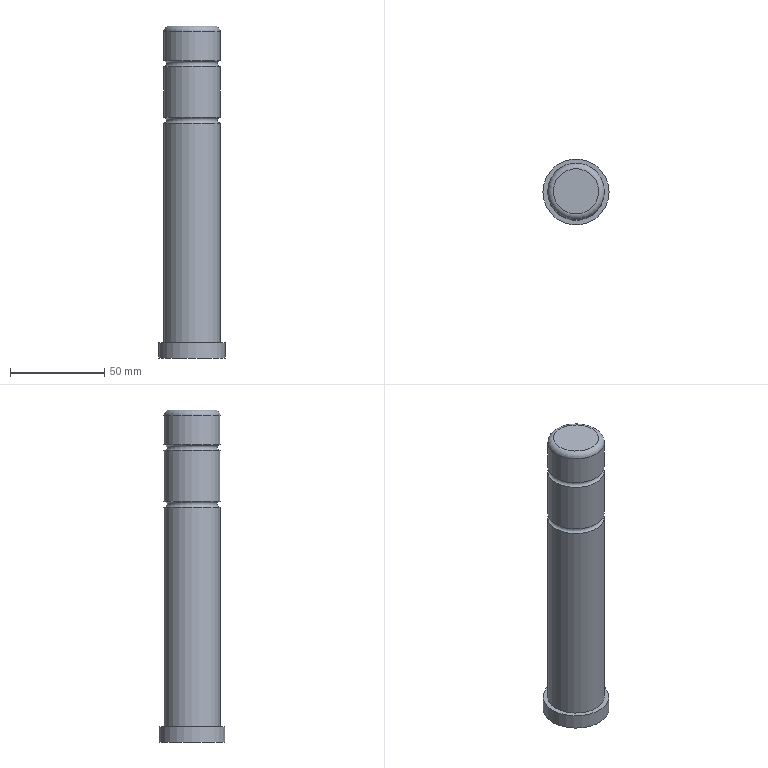Part | NX | features MPPJ 2 | 1 solid | 10 faces | box 35 x 35 x 176 mm | volume 125637 mm3 | cylinder 4 | plane 3 | torus 3 | commonest cylinder face diameters 30 x3 35 x1
STEP:
#1=CARTESIAN_POINT('',(157.,142.,44.));
#2=VERTEX_POINT('',#1);
#3=CARTESIAN_POINT('',(142.,142.,44.));
#4=DIRECTION('',(0.,0.,1.));
#5=DIRECTION('',(1.,0.,0.));
#6=AXIS2_PLACEMENT_3D('',#3,#4,#5);
#7=CIRCLE('',#6,15.);
#8=EDGE_CURVE('',#2,#2,#7,.F.);
#9=ORIENTED_EDGE('',*,*,#8,.T.);
#10=EDGE_LOOP('',(#9));
#11=FACE_BOUND('',#10,.T.);
#12=CARTESIAN_POINT('',(127.,142.,17.));
#13=VERTEX_POINT('',#12);
#14=CARTESIAN_POINT('',(142.,142.,17.));
#15=DIRECTION('',(0.,0.,-1.));
#16=DIRECTION('',(-1.,0.,0.));
#17=AXIS2_PLACEMENT_3D('',#14,#15,#16);
#18=CIRCLE('',#17,15.);
#19=EDGE_CURVE('',#13,#13,#18,.F.);
#20=ORIENTED_EDGE('',*,*,#19,.T.);
#21=EDGE_LOOP('',(#20));
#22=FACE_BOUND('',#21,.T.);
#23=CARTESIAN_POINT('',(142.,142.,-110.5));
#24=DIRECTION('',(0.,0.,1.));
#25=DIRECTION('',(1.,0.,0.));
#26=AXIS2_PLACEMENT_3D('',#23,#24,#25);
#27=CYLINDRICAL_SURFACE('',#26,15.);
#28=ADVANCED_FACE('',(#11,#22),#27,.T.);
#29=CARTESIAN_POINT('',(157.,142.,62.5));
#30=VERTEX_POINT('',#29);
#31=CARTESIAN_POINT('',(142.,142.,62.5));
#32=DIRECTION('',(0.,0.,1.));
#33=DIRECTION('',(1.,0.,0.));
#34=AXIS2_PLACEMENT_3D('',#31,#32,#33);
#35=CIRCLE('',#34,15.);
#36=EDGE_CURVE('',#30,#30,#35,.F.);
#37=ORIENTED_EDGE('',*,*,#36,.T.);
#38=EDGE_LOOP('',(#37));
#39=FACE_BOUND('',#38,.T.);
#40=CARTESIAN_POINT('',(127.,142.,47.));
#41=VERTEX_POINT('',#40);
#42=CARTESIAN_POINT('',(142.,142.,47.));
#43=DIRECTION('',(0.,0.,-1.));
#44=DIRECTION('',(-1.,0.,0.));
#45=AXIS2_PLACEMENT_3D('',#42,#43,#44);
#46=CIRCLE('',#45,15.);
#47=EDGE_CURVE('',#41,#41,#46,.F.);
#48=ORIENTED_EDGE('',*,*,#47,.T.);
#49=EDGE_LOOP('',(#48));
#50=FACE_BOUND('',#49,.T.);
#51=CARTESIAN_POINT('',(142.,142.,-110.5));
#52=DIRECTION('',(0.,0.,1.));
#53=DIRECTION('',(1.,0.,0.));
#54=AXIS2_PLACEMENT_3D('',#51,#52,#53);
#55=CYLINDRICAL_SURFACE('',#54,15.);
#56=ADVANCED_FACE('',(#39,#50),#55,.T.);
#57=CARTESIAN_POINT('',(154.,142.,65.5));
#58=VERTEX_POINT('',#57);
#59=CARTESIAN_POINT('',(142.,142.,65.5));
#60=DIRECTION('',(0.,0.,1.));
#61=DIRECTION('',(1.,0.,0.));
#62=AXIS2_PLACEMENT_3D('',#59,#60,#61);
#63=CIRCLE('',#62,12.);
#64=EDGE_CURVE('',#58,#58,#63,.T.);
#65=ORIENTED_EDGE('',*,*,#64,.T.);
#66=EDGE_LOOP('',(#65));
#67=FACE_BOUND('',#66,.T.);
#68=CARTESIAN_POINT('',(142.,142.,65.5));
#69=DIRECTION('',(0.,0.,1.));
#70=DIRECTION('',(1.,0.,0.));
#71=AXIS2_PLACEMENT_3D('',#68,#69,#70);
#72=PLANE('',#71);
#73=ADVANCED_FACE('',(#67),#72,.T.);
#74=ORIENTED_EDGE('',*,*,#47,.F.);
#75=EDGE_LOOP('',(#74));
#76=FACE_BOUND('',#75,.T.);
#77=ORIENTED_EDGE('',*,*,#8,.F.);
#78=EDGE_LOOP('',(#77));
#79=FACE_BOUND('',#78,.T.);
#80=CARTESIAN_POINT('',(142.,142.,45.5));
#81=DIRECTION('',(0.,0.,1.));
#82=DIRECTION('',(1.,0.,0.));
#83=AXIS2_PLACEMENT_3D('',#80,#81,#82);
#84=TOROIDAL_SURFACE('',#83,15.,1.5);
#85=ADVANCED_FACE('',(#76,#79),#84,.F.);
#86=ORIENTED_EDGE('',*,*,#19,.F.);
#87=EDGE_LOOP('',(#86));
#88=FACE_BOUND('',#87,.T.);
#89=CARTESIAN_POINT('',(157.,142.,14.));
#90=VERTEX_POINT('',#89);
#91=CARTESIAN_POINT('',(142.,142.,14.));
#92=DIRECTION('',(0.,0.,1.));
#93=DIRECTION('',(1.,0.,0.));
#94=AXIS2_PLACEMENT_3D('',#91,#92,#93);
#95=CIRCLE('',#94,15.);
#96=EDGE_CURVE('',#90,#90,#95,.F.);
#97=ORIENTED_EDGE('',*,*,#96,.F.);
#98=EDGE_LOOP('',(#97));
#99=FACE_BOUND('',#98,.T.);
#100=CARTESIAN_POINT('',(142.,142.,15.5));
#101=DIRECTION('',(0.,0.,1.));
#102=DIRECTION('',(1.,0.,0.));
#103=AXIS2_PLACEMENT_3D('',#100,#101,#102);
#104=TOROIDAL_SURFACE('',#103,15.,1.5);
#105=ADVANCED_FACE('',(#88,#99),#104,.F.);
#106=CARTESIAN_POINT('',(157.,142.,-102.5));
#107=VERTEX_POINT('',#106);
#108=CARTESIAN_POINT('',(142.,142.,-102.5));
#109=DIRECTION('',(0.,0.,1.));
#110=DIRECTION('',(1.,0.,0.));
#111=AXIS2_PLACEMENT_3D('',#108,#109,#110);
#112=CIRCLE('',#111,15.);
#113=EDGE_CURVE('',#107,#107,#112,.F.);
#114=ORIENTED_EDGE('',*,*,#113,.F.);
#115=EDGE_LOOP('',(#114));
#116=FACE_BOUND('',#115,.T.);
#117=ORIENTED_EDGE('',*,*,#96,.T.);
#118=EDGE_LOOP('',(#117));
#119=FACE_BOUND('',#118,.T.);
#120=CARTESIAN_POINT('',(142.,142.,-110.5));
#121=DIRECTION('',(0.,0.,1.));
#122=DIRECTION('',(1.,0.,0.));
#123=AXIS2_PLACEMENT_3D('',#120,#121,#122);
#124=CYLINDRICAL_SURFACE('',#123,15.);
#125=ADVANCED_FACE('',(#116,#119),#124,.T.);
#126=ORIENTED_EDGE('',*,*,#113,.T.);
#127=EDGE_LOOP('',(#126));
#128=FACE_BOUND('',#127,.T.);
#129=CARTESIAN_POINT('',(159.5,142.,-102.5));
#130=VERTEX_POINT('',#129);
#131=CARTESIAN_POINT('',(142.,142.,-102.5));
#132=DIRECTION('',(0.,0.,-1.));
#133=DIRECTION('',(1.,0.,0.));
#134=AXIS2_PLACEMENT_3D('',#131,#132,#133);
#135=CIRCLE('',#134,17.5);
#136=EDGE_CURVE('',#130,#130,#135,.T.);
#137=ORIENTED_EDGE('',*,*,#136,.F.);
#138=EDGE_LOOP('',(#137));
#139=FACE_BOUND('',#138,.T.);
#140=CARTESIAN_POINT('',(142.,142.,-102.5));
#141=DIRECTION('',(0.,0.,1.));
#142=DIRECTION('',(1.,0.,0.));
#143=AXIS2_PLACEMENT_3D('',#140,#141,#142);
#144=PLANE('',#143);
#145=ADVANCED_FACE('',(#128,#139),#144,.T.);
#146=ORIENTED_EDGE('',*,*,#136,.T.);
#147=EDGE_LOOP('',(#146));
#148=FACE_BOUND('',#147,.T.);
#149=CARTESIAN_POINT('',(159.5,142.,-110.5));
#150=VERTEX_POINT('',#149);
#151=CARTESIAN_POINT('',(142.,142.,-110.5));
#152=DIRECTION('',(0.,0.,1.));
#153=DIRECTION('',(1.,0.,0.));
#154=AXIS2_PLACEMENT_3D('',#151,#152,#153);
#155=CIRCLE('',#154,17.5);
#156=EDGE_CURVE('',#150,#150,#155,.T.);
#157=ORIENTED_EDGE('',*,*,#156,.T.);
#158=EDGE_LOOP('',(#157));
#159=FACE_BOUND('',#158,.T.);
#160=CARTESIAN_POINT('',(142.,142.,-110.5));
#161=DIRECTION('',(0.,0.,1.));
#162=DIRECTION('',(1.,0.,0.));
#163=AXIS2_PLACEMENT_3D('',#160,#161,#162);
#164=CYLINDRICAL_SURFACE('',#163,17.5);
#165=ADVANCED_FACE('',(#148,#159),#164,.T.);
#166=ORIENTED_EDGE('',*,*,#156,.F.);
#167=EDGE_LOOP('',(#166));
#168=FACE_BOUND('',#167,.T.);
#169=CARTESIAN_POINT('',(142.,142.,-110.5));
#170=DIRECTION('',(0.,0.,-1.));
#171=DIRECTION('',(-1.,0.,0.));
#172=AXIS2_PLACEMENT_3D('',#169,#170,#171);
#173=PLANE('',#172);
#174=ADVANCED_FACE('',(#168),#173,.T.);
#175=ORIENTED_EDGE('',*,*,#64,.F.);
#176=EDGE_LOOP('',(#175));
#177=FACE_BOUND('',#176,.T.);
#178=ORIENTED_EDGE('',*,*,#36,.F.);
#179=EDGE_LOOP('',(#178));
#180=FACE_BOUND('',#179,.T.);
#181=CARTESIAN_POINT('',(142.,142.,62.5));
#182=DIRECTION('',(0.,0.,1.));
#183=DIRECTION('',(1.,0.,0.));
#184=AXIS2_PLACEMENT_3D('',#181,#182,#183);
#185=TOROIDAL_SURFACE('',#184,12.,3.);
#186=ADVANCED_FACE('',(#177,#180),#185,.T.);
#187=CLOSED_SHELL('',(#28,#56,#73,#85,#105,#125,#145,#165,#174,#186));
#188=MANIFOLD_SOLID_BREP('',#187);
#189=(LENGTH_UNIT()NAMED_UNIT(*)SI_UNIT(.MILLI.,.METRE.));
#190=UNCERTAINTY_MEASURE_WITH_UNIT(LENGTH_MEASURE(0.00001),#189,'','');
#191=(NAMED_UNIT(*)PLANE_ANGLE_UNIT()SI_UNIT($,.RADIAN.));
#192=(NAMED_UNIT(*)SI_UNIT($,.STERADIAN.)SOLID_ANGLE_UNIT());
#193=(GEOMETRIC_REPRESENTATION_CONTEXT(3)GLOBAL_UNCERTAINTY_ASSIGNED_CONTEXT((#190))GLOBAL_UNIT_ASSIGNED_CONTEXT((#189,#191,#192))REPRESENTATION_CONTEXT('',''));
#194=ADVANCED_BREP_SHAPE_REPRESENTATION('',(#188),#193);